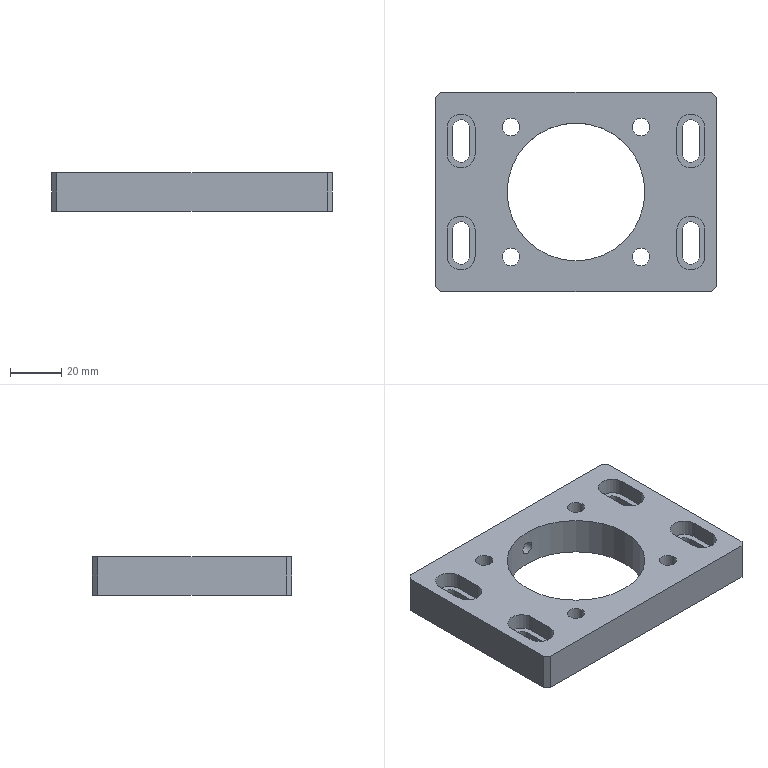CAM job | NX | 3-axis milling, drilling | part box 110 x 78 x 15 mm | stock box 110 x 78 x 15 mm
Tools:
number,name,description,diameter,corner_radius,flute_length,length,flutes
4,D4,平底铣刀-粗,4.0,0.0,25.0,75.0,2
6,D6,平底铣刀-粗,6.0,0.0,25.0,75.0,2
9,D10,平底铣刀-粗,10.0,0.0,35.0,75.0,2
11,D4-J,平底铣刀-精,4.0,0.0,50.0,75.0,2
7,D6-J,平底铣刀-精,6.0,0.0,25.0,75.0,2
10,D10-J,平底铣刀-精,10.0,0.0,35.0,75.0,2
2,D6倒角刀,倒角刀,6.0,0.0,3.0,25.0,2
22,M8X1.25,丝锥,6.8,0.0,35.0,50.0,2
1,C6定点钻,倒角刀,6.0,0.0,3.0,3.0,2
16,ZT6.9,Drilling Tool,6.9,0.0,35.0,50.0,2
Operations:
program,operation,operation_type,tool,method,geometry_group,spindle_rpm,surface_speed,feed_per_tooth,feed_cut,feed_plunge,cut_length_mm,path_length_mm,cut_time_min,machine_time_min
B,选线往复层切开粗-中_COPY_1,PlanarMilling,D10,分层开粗-切深K-步距G,W-B,3000.0,94.245,0.3333,2000.0,100.0,1333.019,2081.381,0.6665,0.7413
B,铣倒角_2,PlanarMilling,D6倒角刀,METHOD,W-B,4000.0,75.398,0.0375,300.0,100.0,95.661,654.373,0.3189,0.3747
B,平面去毛刺6X45L_COPY_1,SurfaceContour,D6倒角刀,爬面_倒角-切深0-步距G,W-B,3500.0,65.972,0.1429,1000.0,100.0,776.265,1343.874,0.7763,0.833
B,平面铣精光侧面-中-直线_COPY_1,PlanarMilling,D10-J,侧刃精光-切深K-步距G,W-B,3000.0,94.245,0.1333,800.0,100.0,67.314,773.071,0.0841,0.1547
A,选线往复层切开粗-中_COPY,PlanarMilling,D10,分层开粗-切深K-步距G,W-A,3000.0,94.245,0.3333,2000.0,100.0,1333.019,2081.381,0.6665,0.7413
A,型腔铣开粗-中_COPY,CavityMilling,D10,分层开粗-切深K-步距G,W-A,3000.0,94.245,0.3333,2000.0,100.0,10753.092,11392.158,5.377,5.473
A,打点-深0.8,Operation,C6定点钻,NONE,W-A,3000.0,56.0,0.01,60.0,90.0,9.0,295.871,0.15,0.1787
A,通孔-M8螺纹底孔,Operation,ZT6.9,NONE,W-A,600.0,12.818,0.1,120.0,90.0,96.0,447.764,0.8,0.8352
A,盲腰槽粗,VolumeBased25DMillingOperation,D6,METHOD,W-A,3500.0,113.0,0.2083,800.0,100.0,4075.336,4670.737,5.094,5.154
A,通腰槽粗_1,VolumeBased25DMillingOperation,D4,METHOD,W-A,3000.0,37.699,0.2,1200.0,100.0,6835.975,7488.976,5.697,5.762
A,腰槽精,VolumeBased25DMillingOperation,D6-J,METHOD,W-A,3200.0,32.0,0.1143,600.0,100.0,303.49,960.192,0.5058,0.5715
A,腰槽精_3,VolumeBased25DMillingOperation,D4-J,METHOD,W-A,3200.0,32.0,0.0781,500.0,100.0,243.172,975.073,0.4863,0.5595
A,铣倒角_1,PlanarMilling,D6倒角刀,METHOD,W-A,4000.0,75.398,0.0625,500.0,100.0,93.908,651.82,0.1878,0.2436
A,平面去毛刺6X45L_COPY,SurfaceContour,D6倒角刀,爬面_倒角-切深0-步距G,W-A,3500.0,65.972,0.1429,1000.0,100.0,831.557,1396.276,0.8316,0.888
A,通孔-攻牙M8,Operation,M8X1.25,METHOD,W-A,300.0,6.409,0.0021,1.25,90.0,82.0,419.764,65.6,65.634
A,平面铣精光侧面-中-直线_COPY,PlanarMilling,D10-J,侧刃精光-切深K-步距G,W-A,3000.0,94.245,0.1333,800.0,100.0,67.314,773.071,0.0841,0.1547
A,底壁铣精光侧面-中_COPY,VolumeBased25DMillingOperation,D10-J,侧刃精光-切深K-步距G,W-A,3000.0,94.245,0.1333,800.0,100.0,294.019,341.74,0.3675,0.3723
A,底壁铣精光侧面-中_COPY_COPY,VolumeBased25DMillingOperation,D10-J,侧刃精光-切深K-步距G,W-A,3000.0,94.245,0.1333,800.0,100.0,294.019,341.74,0.3675,0.3723